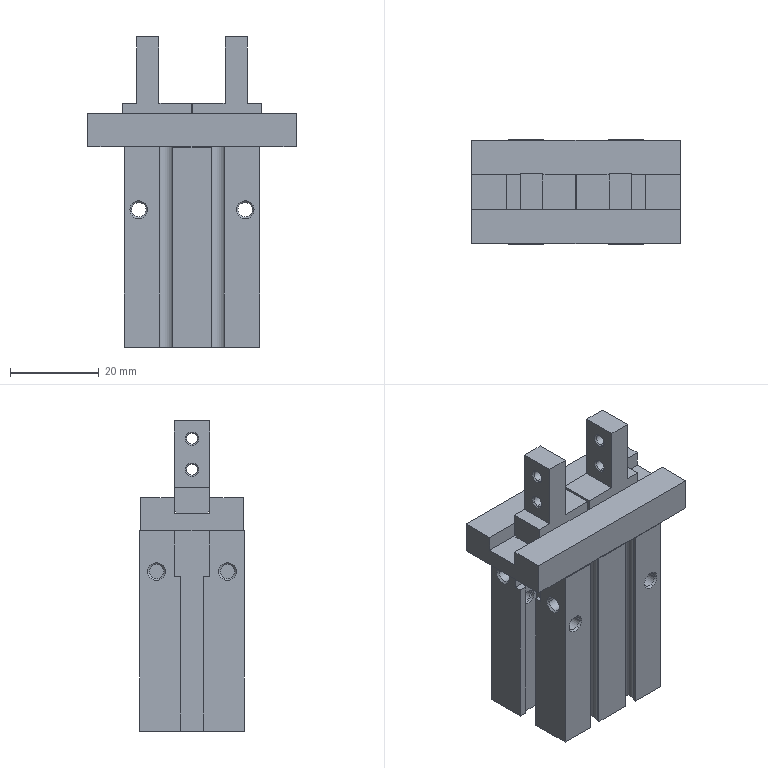Part | STEP file | finger cylinder MHZL2-16D | 3 solids | 222 faces | box 47 x 23.6 x 70 mm | volume 34913 mm3 | plane 126 | cylinder 52 | cone 44 | commonest cylinder face diameters 3.242 x16 2.459 x8 3.4 x8 4 x8 3 x6 4.134 x4